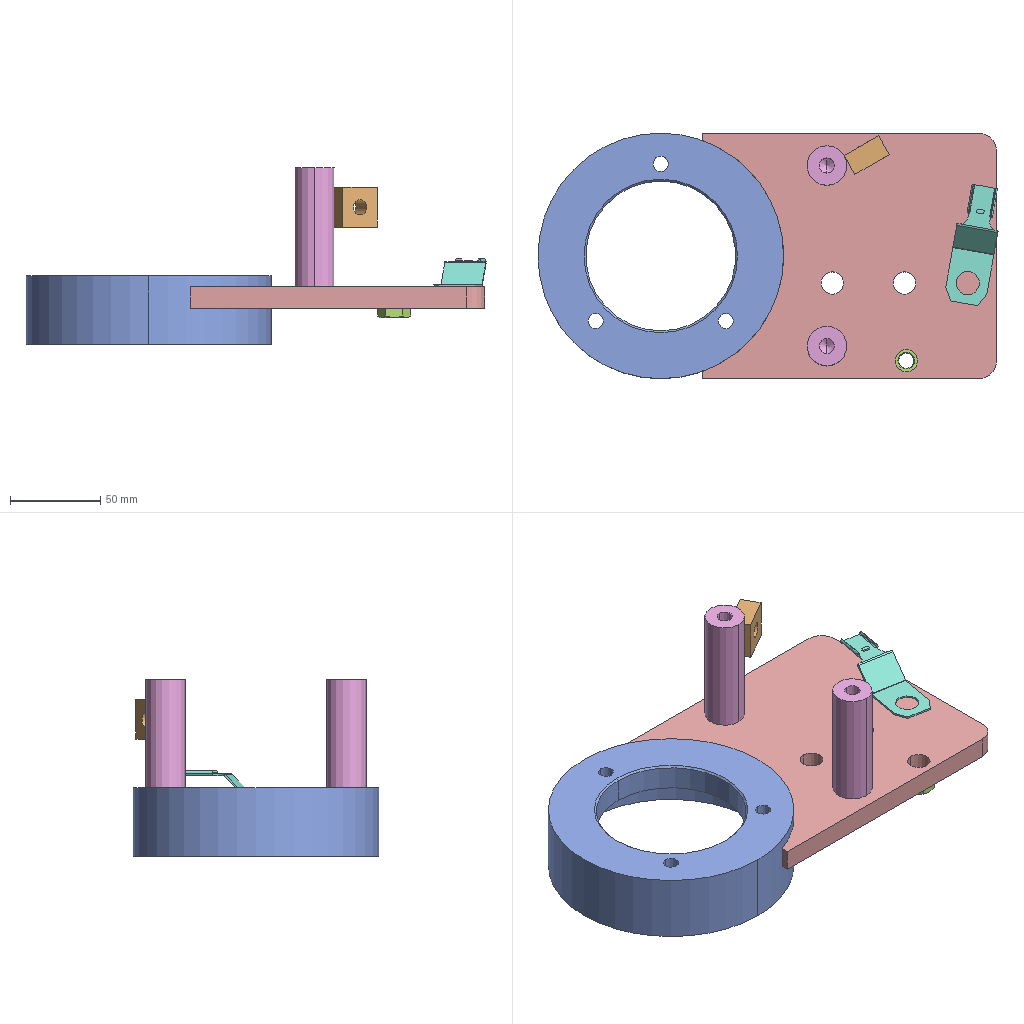Assembly | SolidWorks | 8 different items | 9 placed | box 255 x 136 x 98 mm
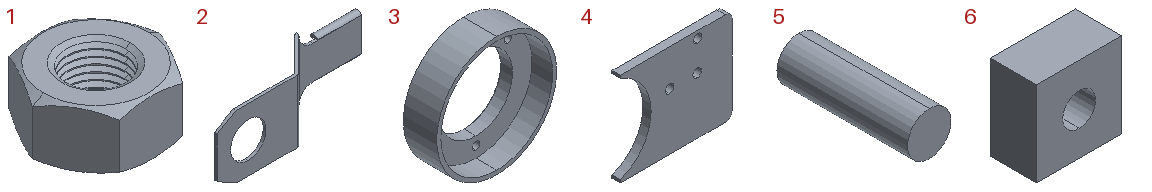Parts list (item | name | quantity | size | volume | features):
1 | - | x1 | 18.475 x 16 x 8.4 mm | 1305 mm3 | features RevCut 2, Chamfer 1, Extrusion 1, LPattern 1
2 | - | x1 | 65.7 x 15.573 x 23.06 mm | 1342 mm3 | features BaseBody 1
3 | - | x1 | 136 x 38 x 136 mm | 173271 mm3 | features Chamfer 1, FlatPattern 1, HoleWzd 1, ICE 1, SMBaseFlange 1, SheetMetal 1
4 | - | x1 | 163 x 12 x 136 mm | 210730 mm3 | features FlatPattern 1, SMBaseFlange 1, SheetMetal 1
5 | - | x2 | 22 x 66 x 22 mm | 23622 mm3 | features Extrusion 1, HoleWzd 1
6 | - | x1 | 22 x 12 x 22 mm | 5127 mm3 | features FlatPattern 1, HoleWzd 1, SMBaseFlange 1, SheetMetal 1
7 | hex nuts, style 1-grades ab gb | x1 | - | - | -
8 | hex nuts, style 1-grades ab gb6 | x1 | - | - | -
Mates (type | each side: item.copy, entity, surface, feature):
Concentric | 4.1 face cylinder Base-Flange1 | 3.1 face cylinder Base-Flange1
DistanceDim | 4.1 face plane Base-Flange1 | 3.1 face plane Base-Flange1
Parallel | 3.1 plane | assembly plane
Coincident | 4.1 face plane Base-Flange1 | 5.1 face plane Boss-Extrude1
DistanceDim | 5.1 plane | 3.1 plane
DistanceDim | 3.1 plane | 5.1 plane
Coincident | 4.1 face plane Base-Flange1 | 2.1 face plane Input1
PlanarAngleDim | 2.1 face plane Input1 | 4.1 face plane Base-Flange1
DistanceDim | 2.1 face cylinder Input1 | 4.1 face plane Base-Flange1
DistanceDim | 4.1 face plane Base-Flange1 | 2.1 face cylinder Input1
PlanarAngleDim | 6.1 face plane Base-Flange1 | 4.1 face plane Base-Flange1
Tangent | 5.2 face cylinder Boss-Extrude1 | 6.1 face plane Base-Flange1
DistanceDim | 6.1 face cylinder M10 Tapped Hole1 | 4.1 face plane Base-Flange1
DistanceDim | 6.1 face plane Base-Flange1 | 5.2 face cylinder M10 Tapped Hole1